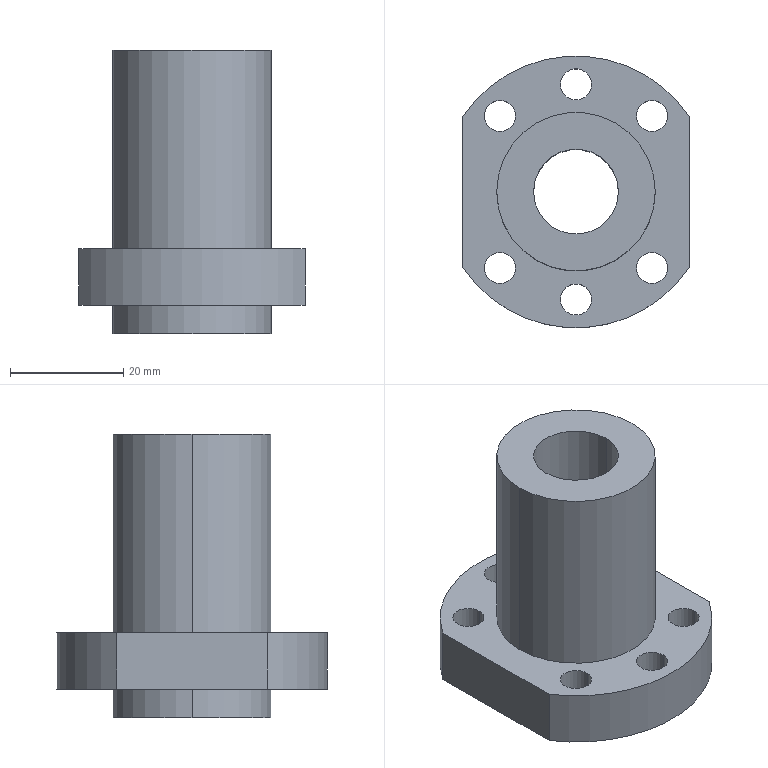Part | STEP file | ball spline SFS01620-1.8 | 1 solid | 26 faces | box 40 x 48 x 50 mm | volume 31024 mm3 | cylinder 20 | plane 6 | commonest cylinder face diameters 5.5 x12 28 x4 15 x2 48 x2